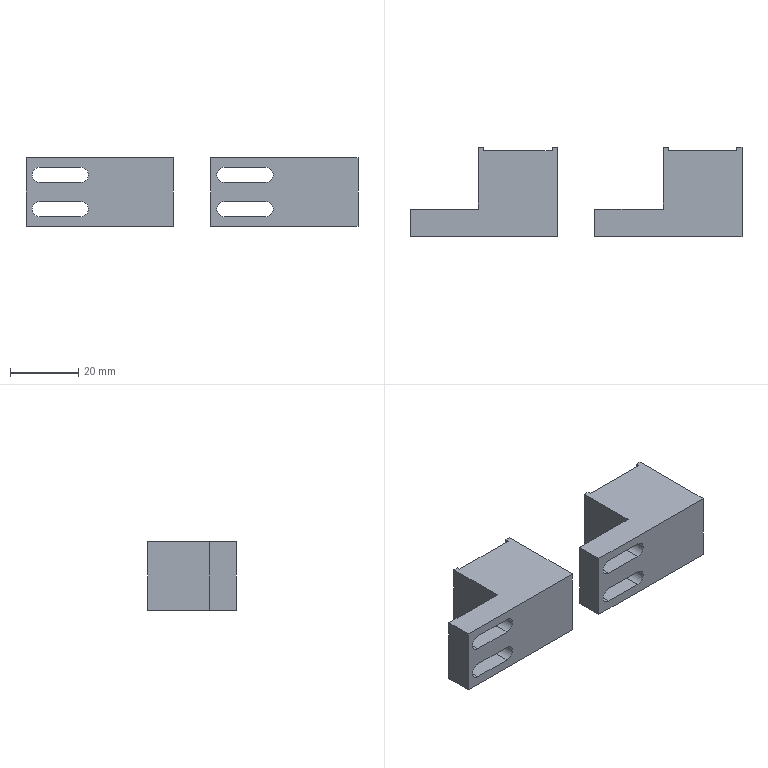CAM job | NX | 3+2 milling, drilling | part box 97 x 26 x 20 mm | stock box 101 x 30 x 25 mm
Tools:
number,name,description,diameter,corner_radius,flute_length,length,flutes
4,D4,平底铣刀-粗,4.0,0.0,25.0,75.0,2
9,D10,平底铣刀-粗,10.0,0.0,35.0,75.0,2
11,D4-J,平底铣刀-精,4.0,0.0,50.0,75.0,2
10,D10-J,平底铣刀-精,10.0,0.0,35.0,75.0,2
1,D80R0.8飞刀,圆鼻刀-粗,80.0,0.8,50.0,75.0,2
1,D80R0.8飞刀-J,圆鼻刀-精,80.0,0.8,50.0,75.0,2
2,D6倒角刀,倒角刀,6.0,0.0,3.0,25.0,2
21,M4X0.7,丝锥,3.3,0.0,35.0,50.0,2
13,钻头3.3,Twist Drill 3.3 mm,3.3,0.0,35.0,35.008,2
Operations:
program,operation,operation_type,tool,method,geometry_group,spindle_rpm,surface_speed,feed_per_tooth,feed_cut,feed_plunge,cut_length_mm,path_length_mm,cut_time_min,machine_time_min
B,底壁铣飞面一刀开粗_COPY,VolumeBased25DMillingOperation,D80R0.8飞刀,分层开粗-切深K-步距G,W-B,2800.0,703.696,0.5357,3000.0,100.0,1641.552,3217.699,0.5472,0.7048
B,底壁铣飞面一刀精光_COPY,VolumeBased25DMillingOperation,D80R0.8飞刀-J,侧刃精光-切深K-步距G,W-B,4000.0,1005.28,0.125,1000.0,100.0,204.998,240.998,0.205,0.2086
B,底壁铣分层开粗-中_COPY,VolumeBased25DMillingOperation,D10,分层开粗-切深K-步距G,W-B,8000.0,251.327,0.3125,5000.0,100.0,6791.586,9198.542,1.358,1.599
B,底壁铣分层开粗-中_COPY_1,VolumeBased25DMillingOperation,D10,分层开粗-切深K-步距G,W-B,8000.0,251.32,0.25,4000.0,100.0,563.803,651.395,0.141,0.1497
B,底壁铣精光底面-中_COPY,VolumeBased25DMillingOperation,D10-J,精光步距切深关,W-B,8000.0,251.32,0.0625,1000.0,100.0,343.242,515.731,0.3432,0.3605
B,底壁铣精光底面-中_COPY_1,VolumeBased25DMillingOperation,D10-J,精光步距切深关,W-B,8000.0,251.32,0.0625,1000.0,100.0,221.702,312.78,0.2217,0.2308
B,打点-深0.8,Operation,D6倒角刀,NONE,W-B,8000.0,150.796,0.0312,500.0,90.0,7.2,123.511,0.0144,0.026
B,盲锥孔-M4螺纹底孔,Operation,钻头3.3,NONE,W-B,3000.0,31.102,0.0417,250.0,90.0,48.366,205.843,0.1935,0.2092
B,钻倒角_1,Operation,D6倒角刀,METHOD,W-B,8000.0,150.796,0.0312,500.0,0.0,20.8,157.583,0.0416,0.0553
B,平面去毛刺6X45L_COPY,SurfaceContour,D6倒角刀,爬面_倒角-切深0-步距G,W-B,6500.0,122.519,0.1154,1500.0,100.0,781.752,1370.245,0.5212,0.58
B,盲锥孔-攻牙M4,Operation,M4X0.7,METHOD,W-B,800.0,8.294,0.0004,0.7,90.0,36.4,181.911,52.0,52.015
B,底壁铣精光侧面-中-选底面_COPY,VolumeBased25DMillingOperation,D10-J,侧刃精光-切深K-步距G,W-B,8000.0,251.32,0.0625,1000.0,100.0,77.364,264.377,0.0774,0.0961
B,底壁铣精光侧面-中-选底面_COPY_1,VolumeBased25DMillingOperation,D10-J,侧刃精光-切深K-步距G,W-B,8000.0,251.32,0.0625,1000.0,100.0,160.885,279.906,0.1609,0.1728
A,顶面,FaceMilling,D80R0.8飞刀,侧刃精光-切深K-步距G,W-A,5000.0,1256.637,0.1,1000.0,100.0,191.0,227.0,0.191,0.1946
A,外形粗_2,VolumeBased25DMillingOperation,D10,METHOD,W-A,8000.0,251.327,0.3125,5000.0,80.0,11066.231,11250.331,2.213,2.232
A,通腰槽粗_1,VolumeBased25DMillingOperation,D4,METHOD,W-A,6000.0,75.398,0.125,1500.0,100.0,3697.667,3961.402,2.465,2.491
A,腰槽精_1,VolumeBased25DMillingOperation,D4-J,METHOD,W-A,6000.0,113.0,0.05,600.0,100.0,222.393,562.444,0.3707,0.4047
A,仅选体,SurfaceContour,D6倒角刀,METHOD,W-A,8000.0,150.796,0.1875,3000.0,100.0,443.07,716.736,0.1477,0.1751
A,外形半精_2,VolumeBased25DMillingOperation,D10-J,METHOD,W-A,8000.0,251.327,0.0625,1000.0,100.0,657.734,976.948,0.6577,0.6897